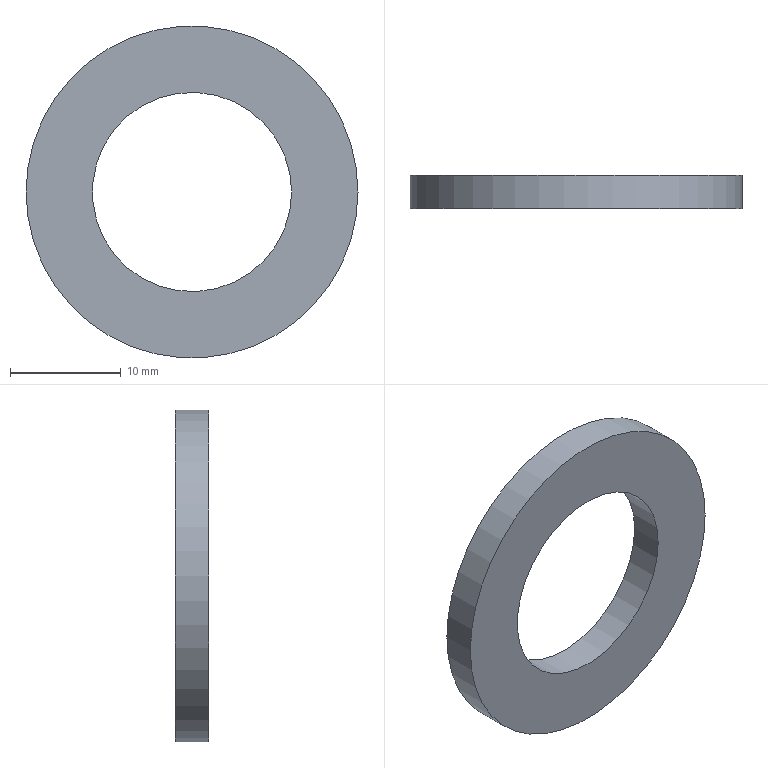Part | NX | features DATUM_CSYS 2, EXTRUDE 1, SKETCH 1 | 1 solid | 4 faces | box 30 x 3 x 30 mm | volume 1357 mm3 | cylinder 2 | plane 2 | commonest cylinder face diameters 18 x1 30 x1
STEP:
#1=CARTESIAN_POINT('',(15.,-3.,0.));
#2=VERTEX_POINT('',#1);
#3=CARTESIAN_POINT('',(0.,-3.,0.));
#4=DIRECTION('',(0.,-1.,0.));
#5=DIRECTION('',(1.,0.,0.));
#6=AXIS2_PLACEMENT_3D('',#3,#4,#5);
#7=CIRCLE('',#6,15.);
#8=EDGE_CURVE('',#2,#2,#7,.T.);
#9=ORIENTED_EDGE('',*,*,#8,.F.);
#10=EDGE_LOOP('',(#9));
#11=FACE_BOUND('',#10,.T.);
#12=CARTESIAN_POINT('',(15.,0.,0.));
#13=VERTEX_POINT('',#12);
#14=CARTESIAN_POINT('',(0.,0.,0.));
#15=DIRECTION('',(0.,-1.,0.));
#16=DIRECTION('',(1.,0.,0.));
#17=AXIS2_PLACEMENT_3D('',#14,#15,#16);
#18=CIRCLE('',#17,15.);
#19=EDGE_CURVE('',#13,#13,#18,.T.);
#20=ORIENTED_EDGE('',*,*,#19,.T.);
#21=EDGE_LOOP('',(#20));
#22=FACE_BOUND('',#21,.T.);
#23=CARTESIAN_POINT('',(0.,-3.,0.));
#24=DIRECTION('',(0.,1.,0.));
#25=DIRECTION('',(0.,0.,1.));
#26=AXIS2_PLACEMENT_3D('',#23,#24,#25);
#27=CYLINDRICAL_SURFACE('',#26,15.);
#28=ADVANCED_FACE('',(#11,#22),#27,.T.);
#29=CARTESIAN_POINT('',(9.,-3.,0.));
#30=VERTEX_POINT('',#29);
#31=CARTESIAN_POINT('',(0.,-3.,0.));
#32=DIRECTION('',(0.,-1.,0.));
#33=DIRECTION('',(1.,0.,0.));
#34=AXIS2_PLACEMENT_3D('',#31,#32,#33);
#35=CIRCLE('',#34,9.);
#36=EDGE_CURVE('',#30,#30,#35,.T.);
#37=ORIENTED_EDGE('',*,*,#36,.T.);
#38=EDGE_LOOP('',(#37));
#39=FACE_BOUND('',#38,.T.);
#40=CARTESIAN_POINT('',(9.,0.,0.));
#41=VERTEX_POINT('',#40);
#42=CARTESIAN_POINT('',(0.,0.,0.));
#43=DIRECTION('',(0.,-1.,0.));
#44=DIRECTION('',(1.,0.,0.));
#45=AXIS2_PLACEMENT_3D('',#42,#43,#44);
#46=CIRCLE('',#45,9.);
#47=EDGE_CURVE('',#41,#41,#46,.T.);
#48=ORIENTED_EDGE('',*,*,#47,.F.);
#49=EDGE_LOOP('',(#48));
#50=FACE_BOUND('',#49,.T.);
#51=CARTESIAN_POINT('',(0.,-3.,0.));
#52=DIRECTION('',(0.,1.,0.));
#53=DIRECTION('',(0.,0.,1.));
#54=AXIS2_PLACEMENT_3D('',#51,#52,#53);
#55=CYLINDRICAL_SURFACE('',#54,9.);
#56=ADVANCED_FACE('',(#39,#50),#55,.F.);
#57=ORIENTED_EDGE('',*,*,#8,.T.);
#58=EDGE_LOOP('',(#57));
#59=FACE_BOUND('',#58,.T.);
#60=ORIENTED_EDGE('',*,*,#36,.F.);
#61=EDGE_LOOP('',(#60));
#62=FACE_BOUND('',#61,.T.);
#63=CARTESIAN_POINT('',(0.,-3.,0.));
#64=DIRECTION('',(0.,-1.,0.));
#65=DIRECTION('',(0.,0.,-1.));
#66=AXIS2_PLACEMENT_3D('',#63,#64,#65);
#67=PLANE('',#66);
#68=ADVANCED_FACE('',(#59,#62),#67,.T.);
#69=ORIENTED_EDGE('',*,*,#19,.F.);
#70=EDGE_LOOP('',(#69));
#71=FACE_BOUND('',#70,.T.);
#72=ORIENTED_EDGE('',*,*,#47,.T.);
#73=EDGE_LOOP('',(#72));
#74=FACE_BOUND('',#73,.T.);
#75=CARTESIAN_POINT('',(0.,0.,0.));
#76=DIRECTION('',(0.,-1.,0.));
#77=DIRECTION('',(0.,0.,-1.));
#78=AXIS2_PLACEMENT_3D('',#75,#76,#77);
#79=PLANE('',#78);
#80=ADVANCED_FACE('',(#71,#74),#79,.F.);
#81=CLOSED_SHELL('',(#28,#56,#68,#80));
#82=MANIFOLD_SOLID_BREP('',#81);
#83=(LENGTH_UNIT()NAMED_UNIT(*)SI_UNIT(.MILLI.,.METRE.));
#84=UNCERTAINTY_MEASURE_WITH_UNIT(LENGTH_MEASURE(0.00001),#83,'','');
#85=(NAMED_UNIT(*)PLANE_ANGLE_UNIT()SI_UNIT($,.RADIAN.));
#86=(NAMED_UNIT(*)SI_UNIT($,.STERADIAN.)SOLID_ANGLE_UNIT());
#87=(GEOMETRIC_REPRESENTATION_CONTEXT(3)GLOBAL_UNCERTAINTY_ASSIGNED_CONTEXT((#84))GLOBAL_UNIT_ASSIGNED_CONTEXT((#83,#85,#86))REPRESENTATION_CONTEXT('',''));
#88=ADVANCED_BREP_SHAPE_REPRESENTATION('',(#82),#87);